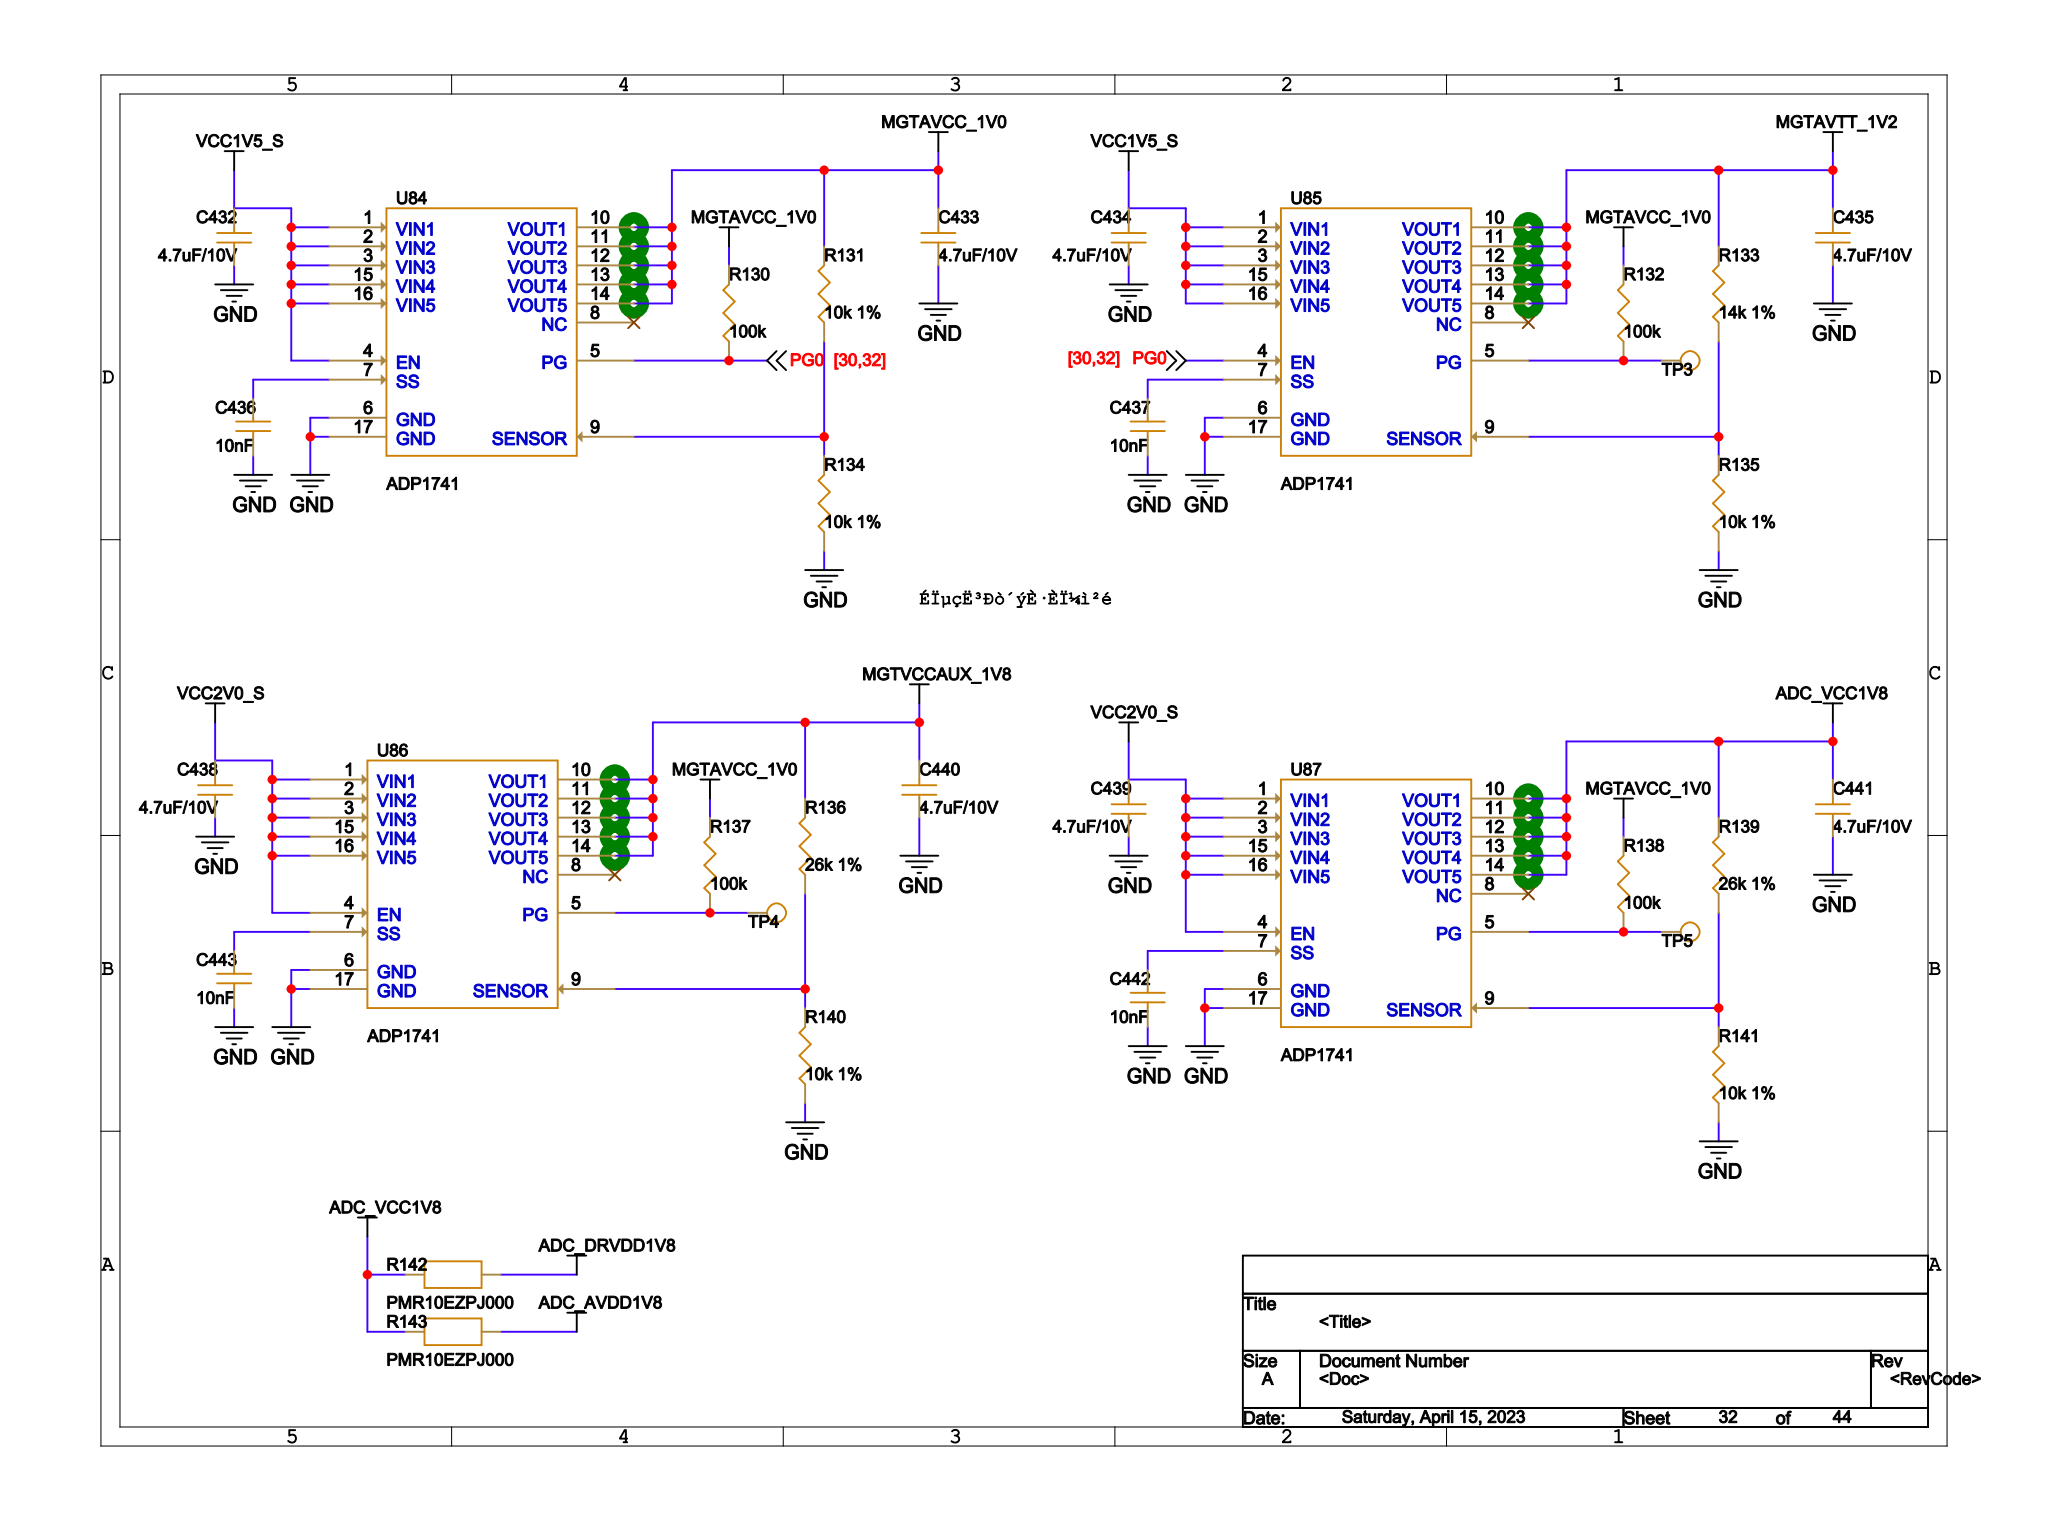Circuit board | Cadence Allegro | 1034 parts | 912 nets | one sheet of the schematic
Parts on this sheet (reference | value | footprint):
C432 | 4.7uF/10V | C0402
C433 | 4.7uF/10V | C0402
C434 | 4.7uF/10V | C0402
C435 | 4.7uF/10V | C0402
C436 | 10nF | C0402
C437 | 10nF | C0402
C438 | 4.7uF/10V | C0402
C439 | 4.7uF/10V | C0402
C440 | 4.7uF/10V | C0402
C441 | 4.7uF/10V | C0402
C442 | 10nF | C0402
C443 | 10nF | C0402
R130 | 100k | R0402
R131 | 10k 1% | R0402
R132 | 100k | R0402
R133 | 14k 1% | R0402
R134 | 10k 1% | R0402
R135 | 10k 1% | R0402
R136 | 26k 1% | R0402
R137 | 100k | R0402
R138 | 100k | R0402
R139 | 26k 1% | R0402
R140 | 10k 1% | R0402
R141 | 10k 1% | R0402
R142 | PMR10EZPJ000 | PMR0805
R143 | PMR10EZPJ000 | PMR0805
TP3 | T POINT R | SMD_M3
TP4 | T POINT R | SMD_M3
TP5 | T POINT R | SMD_M3
U84 | ADP1741 | ADP1741_LFCSP
U85 | ADP1741 | ADP1741_LFCSP
U86 | ADP1741 | ADP1741_LFCSP
U87 | ADP1741 | ADP1741_LFCSP
Nets of these parts (net: part-pin ...):
GND: C432-1 C433-1 C434-1 C435-1 C436-2 C437-2 C438-1 C439-1 C440-1 C441-1 C442-2 C443-2 R134-1 R135-1 R140-1 R141-1 U84-6 U84-17 U85-6 U85-17 U86-6 U86-17 U87-6 U87-17
MGTAVTT_1V2: C435-2 R133-2 U85-10 U85-11 U85-12 U85-13 U85-14
MGTAVCC_1V0: C433-2 R130-2 R131-2 R132-2 R137-2 R138-2 U84-10 U84-11 U84-12 U84-13 U84-14
MGTVCCAUX_1V8: C440-2 R136-2 U86-10 U86-11 U86-12 U86-13 U86-14
ADC_AVDD1V8: R143-2
ADC_DRVDD1V8: R142-2
N14198131: C436-1 U84-7
N14198139: C437-1 U85-7
N14198941: C442-1 U87-7
N14198921: C443-1 U86-7
VCC1V5_S: C432-2 C434-2 U84-1 U84-2 U84-3 U84-4 U84-15 U84-16 U85-1 U85-2 U85-3 U85-15 U85-16
ADC_VCC1V8: C441-2 R139-2 R142-1 R143-1 U87-10 U87-11 U87-12 U87-13 U87-14
VCC2V0_S: C438-2 C439-2 U86-1 U86-2 U86-3 U86-4 U86-15 U86-16 U87-1 U87-2 U87-3 U87-4 U87-15 U87-16
N14198123: R132-1 TP3-1 U85-5
N14198897: R137-1 TP4-1 U86-5
N14198933: R138-1 TP5-1 U87-5
PG0: R130-1 U84-5 U85-4
N14198077: R131-1 R134-2 U84-9
N14198103: R133-1 R135-2 U85-9
N14198889: R136-1 R140-2 U86-9
N14198917: R139-1 R141-2 U87-9